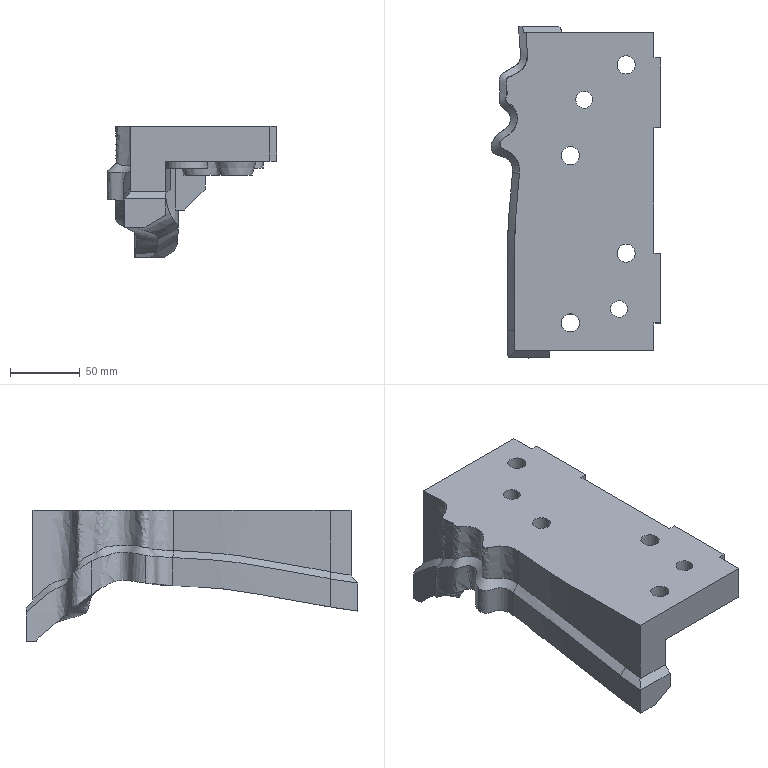Part | NX | features solid 2 | 1 solid | 72 faces | box 121.8 x 238 x 94.152 mm | volume 837135 mm3 | plane 37 | spline 21 | cylinder 12 | cone 2 | commonest cylinder face diameters 13 x6 30 x4 12 x2